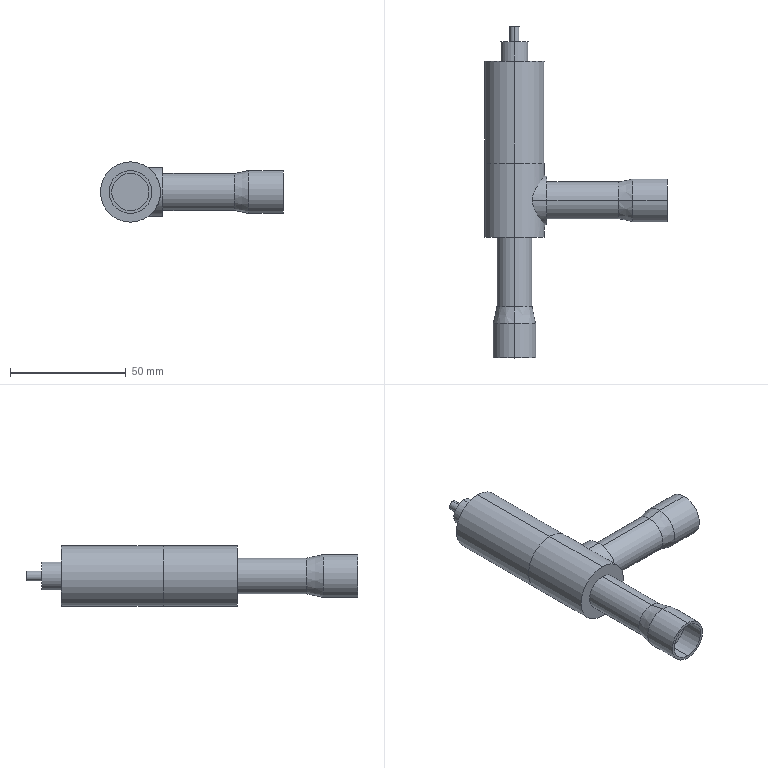Part | STEP file | expansion valve | 3 solids | 42 faces | box 79 x 143.2 x 26 mm | volume 54651 mm3 | cylinder 24 | plane 12 | cone 6 | commonest cylinder face diameters 16.1 x4 18.5 x4 26 x4 4 x2 12 x2 13.6 x2